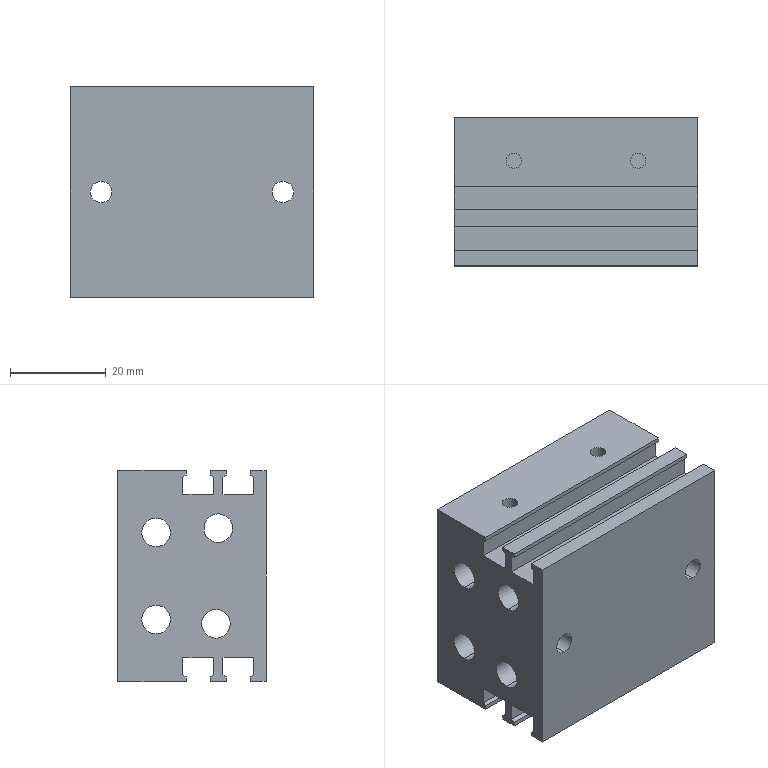Part | SolidWorks | features BaseBody 1 | 1 solid | 94 faces | box 51 x 31 x 44 mm | volume 55685 mm3 | plane 51 | cylinder 35 | cone 8 | commonest cylinder face diameters 3.242 x12 6 x8 3 x5 4.134 x4 4.5 x4 18 x2